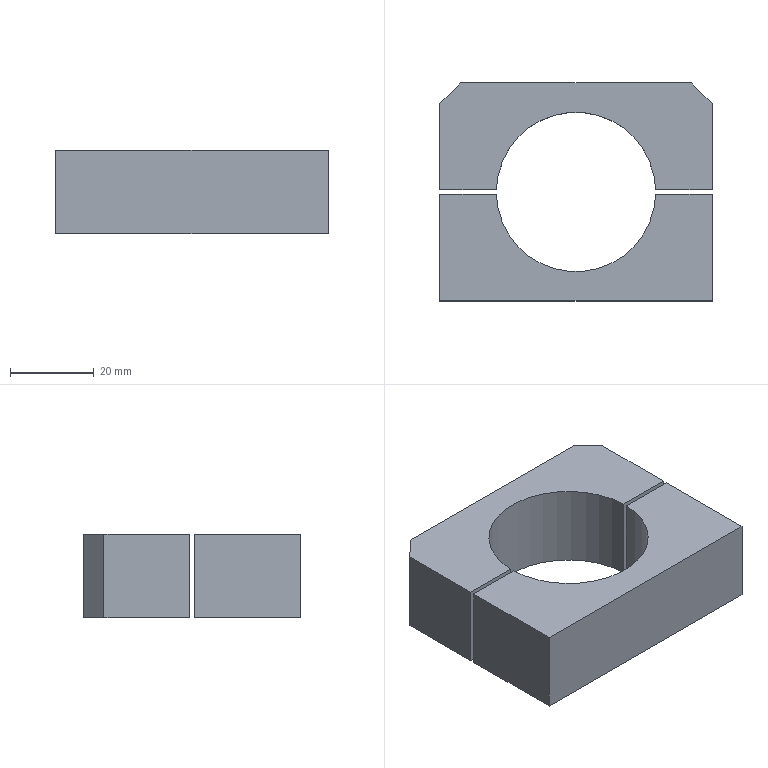Part | STEP file | PN_0008 | 2 solids | 18 faces | box 65 x 52 x 20 mm | volume 43878 mm3 | plane 16 | cylinder 2 | commonest cylinder face diameters 38 x2
STEP:
#1=CARTESIAN_POINT('',(0.,0.,0.));
#2=DIRECTION('',(0.,0.,1.));
#3=DIRECTION('',(1.,0.,0.));
#4=AXIS2_PLACEMENT_3D('',#1,#2,#3);
#5=CARTESIAN_POINT('',(-32.5,-0.5,20.));
#6=VERTEX_POINT('',#5);
#7=CARTESIAN_POINT('',(-18.993,-0.5,20.));
#8=VERTEX_POINT('',#7);
#9=CARTESIAN_POINT('',(-36.358,-0.5,20.));
#10=DIRECTION('',(1.,0.,0.));
#11=VECTOR('',#10,1.);
#12=LINE('',#9,#11);
#13=CARTESIAN_POINT('',(32.5,-26.,20.));
#14=DIRECTION('',(0.,0.,1.));
#15=DIRECTION('',(1.,0.,0.));
#16=AXIS2_PLACEMENT_3D('',#13,#14,#15);
#17=PLANE('',#16);
#18=CARTESIAN_POINT('',(-68.858,25.5));
#19=DIRECTION('',(1.,0.));
#20=VECTOR('',#19,1.);
#21=LINE('',#18,#20);
#22=(GEOMETRIC_REPRESENTATION_CONTEXT(2)PARAMETRIC_REPRESENTATION_CONTEXT()REPRESENTATION_CONTEXT('',''));
#23=DEFINITIONAL_REPRESENTATION('',(#21),#22);
#24=PCURVE('',#17,#23);
#25=CARTESIAN_POINT('',(-36.358,-0.5,0.));
#26=DIRECTION('',(0.,-1.,0.));
#27=DIRECTION('',(0.,0.,-1.));
#28=AXIS2_PLACEMENT_3D('',#25,#26,#27);
#29=PLANE('',#28);
#30=CARTESIAN_POINT('',(-20.,0.));
#31=DIRECTION('',(0.,1.));
#32=VECTOR('',#31,1.);
#33=LINE('',#30,#32);
#34=(GEOMETRIC_REPRESENTATION_CONTEXT(2)PARAMETRIC_REPRESENTATION_CONTEXT()REPRESENTATION_CONTEXT('',''));
#35=DEFINITIONAL_REPRESENTATION('',(#33),#34);
#36=PCURVE('',#29,#35);
#37=SURFACE_CURVE('',#12,(#24,#36),.PCURVE_S1.);
#38=EDGE_CURVE('',#6,#8,#37,.T.);
#39=ORIENTED_EDGE('',*,*,#38,.F.);
#40=CARTESIAN_POINT('',(-32.5,-26.,20.));
#41=VERTEX_POINT('',#40);
#42=CARTESIAN_POINT('',(-32.5,26.,20.));
#43=DIRECTION('',(0.,-1.,0.));
#44=VECTOR('',#43,1.);
#45=LINE('',#42,#44);
#46=CARTESIAN_POINT('',(-65.,52.));
#47=DIRECTION('',(0.,-1.));
#48=VECTOR('',#47,1.);
#49=LINE('',#46,#48);
#50=(GEOMETRIC_REPRESENTATION_CONTEXT(2)PARAMETRIC_REPRESENTATION_CONTEXT()REPRESENTATION_CONTEXT('',''));
#51=DEFINITIONAL_REPRESENTATION('',(#49),#50);
#52=PCURVE('',#17,#51);
#53=CARTESIAN_POINT('',(-32.5,26.,20.));
#54=DIRECTION('',(1.,0.,0.));
#55=DIRECTION('',(0.,1.,0.));
#56=AXIS2_PLACEMENT_3D('',#53,#54,#55);
#57=PLANE('',#56);
#58=CARTESIAN_POINT('',(0.,0.));
#59=DIRECTION('',(-1.,0.));
#60=VECTOR('',#59,1.);
#61=LINE('',#58,#60);
#62=(GEOMETRIC_REPRESENTATION_CONTEXT(2)PARAMETRIC_REPRESENTATION_CONTEXT()REPRESENTATION_CONTEXT('',''));
#63=DEFINITIONAL_REPRESENTATION('',(#61),#62);
#64=PCURVE('',#57,#63);
#65=SURFACE_CURVE('',#45,(#52,#64),.PCURVE_S1.);
#66=EDGE_CURVE('',#6,#41,#65,.T.);
#67=ORIENTED_EDGE('',*,*,#66,.T.);
#68=CARTESIAN_POINT('',(32.5,-26.,20.));
#69=VERTEX_POINT('',#68);
#70=CARTESIAN_POINT('',(-32.5,-26.,20.));
#71=DIRECTION('',(1.,0.,0.));
#72=VECTOR('',#71,1.);
#73=LINE('',#70,#72);
#74=CARTESIAN_POINT('',(-65.,0.));
#75=DIRECTION('',(1.,0.));
#76=VECTOR('',#75,1.);
#77=LINE('',#74,#76);
#78=(GEOMETRIC_REPRESENTATION_CONTEXT(2)PARAMETRIC_REPRESENTATION_CONTEXT()REPRESENTATION_CONTEXT('',''));
#79=DEFINITIONAL_REPRESENTATION('',(#77),#78);
#80=PCURVE('',#17,#79);
#81=CARTESIAN_POINT('',(-32.5,-26.,20.));
#82=DIRECTION('',(0.,1.,0.));
#83=DIRECTION('',(0.,0.,1.));
#84=AXIS2_PLACEMENT_3D('',#81,#82,#83);
#85=PLANE('',#84);
#86=CARTESIAN_POINT('',(0.,0.));
#87=DIRECTION('',(0.,1.));
#88=VECTOR('',#87,1.);
#89=LINE('',#86,#88);
#90=(GEOMETRIC_REPRESENTATION_CONTEXT(2)PARAMETRIC_REPRESENTATION_CONTEXT()REPRESENTATION_CONTEXT('',''));
#91=DEFINITIONAL_REPRESENTATION('',(#89),#90);
#92=PCURVE('',#85,#91);
#93=SURFACE_CURVE('',#73,(#80,#92),.PCURVE_S1.);
#94=EDGE_CURVE('',#41,#69,#93,.T.);
#95=ORIENTED_EDGE('',*,*,#94,.T.);
#96=CARTESIAN_POINT('',(32.5,-0.5,20.));
#97=VERTEX_POINT('',#96);
#98=CARTESIAN_POINT('',(32.5,26.,20.));
#99=DIRECTION('',(0.,1.,0.));
#100=VECTOR('',#99,1.);
#101=LINE('',#98,#100);
#102=CARTESIAN_POINT('',(0.,52.));
#103=DIRECTION('',(0.,1.));
#104=VECTOR('',#103,1.);
#105=LINE('',#102,#104);
#106=(GEOMETRIC_REPRESENTATION_CONTEXT(2)PARAMETRIC_REPRESENTATION_CONTEXT()REPRESENTATION_CONTEXT('',''));
#107=DEFINITIONAL_REPRESENTATION('',(#105),#106);
#108=PCURVE('',#17,#107);
#109=CARTESIAN_POINT('',(32.5,26.,20.));
#110=DIRECTION('',(-1.,0.,0.));
#111=DIRECTION('',(0.,-1.,0.));
#112=AXIS2_PLACEMENT_3D('',#109,#110,#111);
#113=PLANE('',#112);
#114=CARTESIAN_POINT('',(0.,0.));
#115=DIRECTION('',(-1.,0.));
#116=VECTOR('',#115,1.);
#117=LINE('',#114,#116);
#118=(GEOMETRIC_REPRESENTATION_CONTEXT(2)PARAMETRIC_REPRESENTATION_CONTEXT()REPRESENTATION_CONTEXT('',''));
#119=DEFINITIONAL_REPRESENTATION('',(#117),#118);
#120=PCURVE('',#113,#119);
#121=SURFACE_CURVE('',#101,(#108,#120),.PCURVE_S1.);
#122=EDGE_CURVE('',#69,#97,#121,.T.);
#123=ORIENTED_EDGE('',*,*,#122,.T.);
#124=CARTESIAN_POINT('',(18.993,-0.5,20.));
#125=VERTEX_POINT('',#124);
#126=CARTESIAN_POINT('',(-36.358,-0.5,20.));
#127=DIRECTION('',(1.,0.,0.));
#128=VECTOR('',#127,1.);
#129=LINE('',#126,#128);
#130=CARTESIAN_POINT('',(-68.858,25.5));
#131=DIRECTION('',(1.,0.));
#132=VECTOR('',#131,1.);
#133=LINE('',#130,#132);
#134=(GEOMETRIC_REPRESENTATION_CONTEXT(2)PARAMETRIC_REPRESENTATION_CONTEXT()REPRESENTATION_CONTEXT('',''));
#135=DEFINITIONAL_REPRESENTATION('',(#133),#134);
#136=PCURVE('',#17,#135);
#137=CARTESIAN_POINT('',(-36.358,-0.5,0.));
#138=DIRECTION('',(0.,-1.,0.));
#139=DIRECTION('',(0.,0.,-1.));
#140=AXIS2_PLACEMENT_3D('',#137,#138,#139);
#141=PLANE('',#140);
#142=CARTESIAN_POINT('',(-20.,0.));
#143=DIRECTION('',(0.,1.));
#144=VECTOR('',#143,1.);
#145=LINE('',#142,#144);
#146=(GEOMETRIC_REPRESENTATION_CONTEXT(2)PARAMETRIC_REPRESENTATION_CONTEXT()REPRESENTATION_CONTEXT('',''));
#147=DEFINITIONAL_REPRESENTATION('',(#145),#146);
#148=PCURVE('',#141,#147);
#149=SURFACE_CURVE('',#129,(#136,#148),.PCURVE_S1.);
#150=EDGE_CURVE('',#125,#97,#149,.T.);
#151=ORIENTED_EDGE('',*,*,#150,.F.);
#152=CARTESIAN_POINT('',(0.,0.,20.));
#153=DIRECTION('',(0.,0.,1.));
#154=DIRECTION('',(1.,0.,0.));
#155=AXIS2_PLACEMENT_3D('',#152,#153,#154);
#156=CIRCLE('',#155,19.);
#157=CARTESIAN_POINT('',(-32.5,26.));
#158=DIRECTION('',(1.,0.));
#159=AXIS2_PLACEMENT_2D('',#157,#158);
#160=CIRCLE('',#159,19.);
#161=(GEOMETRIC_REPRESENTATION_CONTEXT(2)PARAMETRIC_REPRESENTATION_CONTEXT()REPRESENTATION_CONTEXT('',''));
#162=DEFINITIONAL_REPRESENTATION('',(#160),#161);
#163=PCURVE('',#17,#162);
#164=CARTESIAN_POINT('',(0.,0.,20.));
#165=DIRECTION('',(0.,0.,-1.));
#166=DIRECTION('',(-1.,0.,0.));
#167=AXIS2_PLACEMENT_3D('',#164,#165,#166);
#168=CYLINDRICAL_SURFACE('',#167,19.);
#169=CARTESIAN_POINT('',(9.425,0.));
#170=DIRECTION('',(-1.,0.));
#171=VECTOR('',#170,1.);
#172=LINE('',#169,#171);
#173=(GEOMETRIC_REPRESENTATION_CONTEXT(2)PARAMETRIC_REPRESENTATION_CONTEXT()REPRESENTATION_CONTEXT('',''));
#174=DEFINITIONAL_REPRESENTATION('',(#172),#173);
#175=PCURVE('',#168,#174);
#176=SURFACE_CURVE('',#156,(#163,#175),.PCURVE_S1.);
#177=EDGE_CURVE('',#8,#125,#176,.T.);
#178=ORIENTED_EDGE('',*,*,#177,.F.);
#179=EDGE_LOOP('',(#39,#67,#95,#123,#151,#178));
#180=FACE_BOUND('',#179,.T.);
#181=ADVANCED_FACE('',(#180),#17,.T.);
#182=CARTESIAN_POINT('',(-32.5,-0.5,0.));
#183=VERTEX_POINT('',#182);
#184=CARTESIAN_POINT('',(-32.5,-26.,0.));
#185=VERTEX_POINT('',#184);
#186=CARTESIAN_POINT('',(-32.5,26.,0.));
#187=DIRECTION('',(0.,-1.,0.));
#188=VECTOR('',#187,1.);
#189=LINE('',#186,#188);
#190=CARTESIAN_POINT('',(32.5,-26.,0.));
#191=DIRECTION('',(0.,0.,1.));
#192=DIRECTION('',(1.,0.,0.));
#193=AXIS2_PLACEMENT_3D('',#190,#191,#192);
#194=PLANE('',#193);
#195=CARTESIAN_POINT('',(-65.,52.));
#196=DIRECTION('',(0.,-1.));
#197=VECTOR('',#196,1.);
#198=LINE('',#195,#197);
#199=(GEOMETRIC_REPRESENTATION_CONTEXT(2)PARAMETRIC_REPRESENTATION_CONTEXT()REPRESENTATION_CONTEXT('',''));
#200=DEFINITIONAL_REPRESENTATION('',(#198),#199);
#201=PCURVE('',#194,#200);
#202=CARTESIAN_POINT('',(0.,-20.));
#203=DIRECTION('',(-1.,0.));
#204=VECTOR('',#203,1.);
#205=LINE('',#202,#204);
#206=(GEOMETRIC_REPRESENTATION_CONTEXT(2)PARAMETRIC_REPRESENTATION_CONTEXT()REPRESENTATION_CONTEXT('',''));
#207=DEFINITIONAL_REPRESENTATION('',(#205),#206);
#208=PCURVE('',#57,#207);
#209=SURFACE_CURVE('',#189,(#201,#208),.PCURVE_S1.);
#210=EDGE_CURVE('',#183,#185,#209,.T.);
#211=ORIENTED_EDGE('',*,*,#210,.F.);
#212=CARTESIAN_POINT('',(-18.993,-0.5,0.));
#213=VERTEX_POINT('',#212);
#214=CARTESIAN_POINT('',(-36.358,-0.5,0.));
#215=DIRECTION('',(1.,0.,0.));
#216=VECTOR('',#215,1.);
#217=LINE('',#214,#216);
#218=CARTESIAN_POINT('',(-68.858,25.5));
#219=DIRECTION('',(1.,0.));
#220=VECTOR('',#219,1.);
#221=LINE('',#218,#220);
#222=(GEOMETRIC_REPRESENTATION_CONTEXT(2)PARAMETRIC_REPRESENTATION_CONTEXT()REPRESENTATION_CONTEXT('',''));
#223=DEFINITIONAL_REPRESENTATION('',(#221),#222);
#224=PCURVE('',#194,#223);
#225=CARTESIAN_POINT('',(0.,0.));
#226=DIRECTION('',(0.,1.));
#227=VECTOR('',#226,1.);
#228=LINE('',#225,#227);
#229=(GEOMETRIC_REPRESENTATION_CONTEXT(2)PARAMETRIC_REPRESENTATION_CONTEXT()REPRESENTATION_CONTEXT('',''));
#230=DEFINITIONAL_REPRESENTATION('',(#228),#229);
#231=PCURVE('',#29,#230);
#232=SURFACE_CURVE('',#217,(#224,#231),.PCURVE_S1.);
#233=EDGE_CURVE('',#183,#213,#232,.T.);
#234=ORIENTED_EDGE('',*,*,#233,.T.);
#235=CARTESIAN_POINT('',(18.993,-0.5,0.));
#236=VERTEX_POINT('',#235);
#237=CARTESIAN_POINT('',(0.,0.,0.));
#238=DIRECTION('',(0.,0.,1.));
#239=DIRECTION('',(1.,0.,0.));
#240=AXIS2_PLACEMENT_3D('',#237,#238,#239);
#241=CIRCLE('',#240,19.);
#242=CARTESIAN_POINT('',(-32.5,26.));
#243=DIRECTION('',(1.,0.));
#244=AXIS2_PLACEMENT_2D('',#242,#243);
#245=CIRCLE('',#244,19.);
#246=(GEOMETRIC_REPRESENTATION_CONTEXT(2)PARAMETRIC_REPRESENTATION_CONTEXT()REPRESENTATION_CONTEXT('',''));
#247=DEFINITIONAL_REPRESENTATION('',(#245),#246);
#248=PCURVE('',#194,#247);
#249=CARTESIAN_POINT('',(9.425,20.));
#250=DIRECTION('',(-1.,0.));
#251=VECTOR('',#250,1.);
#252=LINE('',#249,#251);
#253=(GEOMETRIC_REPRESENTATION_CONTEXT(2)PARAMETRIC_REPRESENTATION_CONTEXT()REPRESENTATION_CONTEXT('',''));
#254=DEFINITIONAL_REPRESENTATION('',(#252),#253);
#255=PCURVE('',#168,#254);
#256=SURFACE_CURVE('',#241,(#248,#255),.PCURVE_S1.);
#257=EDGE_CURVE('',#213,#236,#256,.T.);
#258=ORIENTED_EDGE('',*,*,#257,.T.);
#259=CARTESIAN_POINT('',(32.5,-0.5,0.));
#260=VERTEX_POINT('',#259);
#261=CARTESIAN_POINT('',(-36.358,-0.5,0.));
#262=DIRECTION('',(1.,0.,0.));
#263=VECTOR('',#262,1.);
#264=LINE('',#261,#263);
#265=CARTESIAN_POINT('',(-68.858,25.5));
#266=DIRECTION('',(1.,0.));
#267=VECTOR('',#266,1.);
#268=LINE('',#265,#267);
#269=(GEOMETRIC_REPRESENTATION_CONTEXT(2)PARAMETRIC_REPRESENTATION_CONTEXT()REPRESENTATION_CONTEXT('',''));
#270=DEFINITIONAL_REPRESENTATION('',(#268),#269);
#271=PCURVE('',#194,#270);
#272=CARTESIAN_POINT('',(0.,0.));
#273=DIRECTION('',(0.,1.));
#274=VECTOR('',#273,1.);
#275=LINE('',#272,#274);
#276=(GEOMETRIC_REPRESENTATION_CONTEXT(2)PARAMETRIC_REPRESENTATION_CONTEXT()REPRESENTATION_CONTEXT('',''));
#277=DEFINITIONAL_REPRESENTATION('',(#275),#276);
#278=PCURVE('',#141,#277);
#279=SURFACE_CURVE('',#264,(#271,#278),.PCURVE_S1.);
#280=EDGE_CURVE('',#236,#260,#279,.T.);
#281=ORIENTED_EDGE('',*,*,#280,.T.);
#282=CARTESIAN_POINT('',(32.5,-26.,0.));
#283=VERTEX_POINT('',#282);
#284=CARTESIAN_POINT('',(32.5,26.,0.));
#285=DIRECTION('',(0.,1.,0.));
#286=VECTOR('',#285,1.);
#287=LINE('',#284,#286);
#288=CARTESIAN_POINT('',(0.,52.));
#289=DIRECTION('',(0.,1.));
#290=VECTOR('',#289,1.);
#291=LINE('',#288,#290);
#292=(GEOMETRIC_REPRESENTATION_CONTEXT(2)PARAMETRIC_REPRESENTATION_CONTEXT()REPRESENTATION_CONTEXT('',''));
#293=DEFINITIONAL_REPRESENTATION('',(#291),#292);
#294=PCURVE('',#194,#293);
#295=CARTESIAN_POINT('',(0.,-20.));
#296=DIRECTION('',(-1.,0.));
#297=VECTOR('',#296,1.);
#298=LINE('',#295,#297);
#299=(GEOMETRIC_REPRESENTATION_CONTEXT(2)PARAMETRIC_REPRESENTATION_CONTEXT()REPRESENTATION_CONTEXT('',''));
#300=DEFINITIONAL_REPRESENTATION('',(#298),#299);
#301=PCURVE('',#113,#300);
#302=SURFACE_CURVE('',#287,(#294,#301),.PCURVE_S1.);
#303=EDGE_CURVE('',#283,#260,#302,.T.);
#304=ORIENTED_EDGE('',*,*,#303,.F.);
#305=CARTESIAN_POINT('',(-32.5,-26.,0.));
#306=DIRECTION('',(1.,0.,0.));
#307=VECTOR('',#306,1.);
#308=LINE('',#305,#307);
#309=CARTESIAN_POINT('',(-65.,0.));
#310=DIRECTION('',(1.,0.));
#311=VECTOR('',#310,1.);
#312=LINE('',#309,#311);
#313=(GEOMETRIC_REPRESENTATION_CONTEXT(2)PARAMETRIC_REPRESENTATION_CONTEXT()REPRESENTATION_CONTEXT('',''));
#314=DEFINITIONAL_REPRESENTATION('',(#312),#313);
#315=PCURVE('',#194,#314);
#316=CARTESIAN_POINT('',(-20.,0.));
#317=DIRECTION('',(0.,1.));
#318=VECTOR('',#317,1.);
#319=LINE('',#316,#318);
#320=(GEOMETRIC_REPRESENTATION_CONTEXT(2)PARAMETRIC_REPRESENTATION_CONTEXT()REPRESENTATION_CONTEXT('',''));
#321=DEFINITIONAL_REPRESENTATION('',(#319),#320);
#322=PCURVE('',#85,#321);
#323=SURFACE_CURVE('',#308,(#315,#322),.PCURVE_S1.);
#324=EDGE_CURVE('',#185,#283,#323,.T.);
#325=ORIENTED_EDGE('',*,*,#324,.F.);
#326=EDGE_LOOP('',(#211,#234,#258,#281,#304,#325));
#327=FACE_BOUND('',#326,.T.);
#328=ADVANCED_FACE('',(#327),#194,.F.);
#329=ORIENTED_EDGE('',*,*,#303,.T.);
#330=CARTESIAN_POINT('',(32.5,-0.5,20.));
#331=DIRECTION('',(0.,0.,1.));
#332=VECTOR('',#331,1.);
#333=LINE('',#330,#332);
#334=CARTESIAN_POINT('',(26.5,0.));
#335=DIRECTION('',(0.,1.));
#336=VECTOR('',#335,1.);
#337=LINE('',#334,#336);
#338=(GEOMETRIC_REPRESENTATION_CONTEXT(2)PARAMETRIC_REPRESENTATION_CONTEXT()REPRESENTATION_CONTEXT('',''));
#339=DEFINITIONAL_REPRESENTATION('',(#337),#338);
#340=PCURVE('',#113,#339);
#341=CARTESIAN_POINT('',(-20.,68.858));
#342=DIRECTION('',(-1.,0.));
#343=VECTOR('',#342,1.);
#344=LINE('',#341,#343);
#345=(GEOMETRIC_REPRESENTATION_CONTEXT(2)PARAMETRIC_REPRESENTATION_CONTEXT()REPRESENTATION_CONTEXT('',''));
#346=DEFINITIONAL_REPRESENTATION('',(#344),#345);
#347=PCURVE('',#141,#346);
#348=SURFACE_CURVE('',#333,(#340,#347),.PCURVE_S1.);
#349=EDGE_CURVE('',#260,#97,#348,.T.);
#350=ORIENTED_EDGE('',*,*,#349,.T.);
#351=ORIENTED_EDGE('',*,*,#122,.F.);
#352=CARTESIAN_POINT('',(32.5,-26.,20.));
#353=DIRECTION('',(0.,0.,-1.));
#354=VECTOR('',#353,1.);
#355=LINE('',#352,#354);
#356=CARTESIAN_POINT('',(52.,0.));
#357=DIRECTION('',(0.,-1.));
#358=VECTOR('',#357,1.);
#359=LINE('',#356,#358);
#360=(GEOMETRIC_REPRESENTATION_CONTEXT(2)PARAMETRIC_REPRESENTATION_CONTEXT()REPRESENTATION_CONTEXT('',''));
#361=DEFINITIONAL_REPRESENTATION('',(#359),#360);
#362=PCURVE('',#113,#361);
#363=CARTESIAN_POINT('',(0.,65.));
#364=DIRECTION('',(-1.,0.));
#365=VECTOR('',#364,1.);
#366=LINE('',#363,#365);
#367=(GEOMETRIC_REPRESENTATION_CONTEXT(2)PARAMETRIC_REPRESENTATION_CONTEXT()REPRESENTATION_CONTEXT('',''));
#368=DEFINITIONAL_REPRESENTATION('',(#366),#367);
#369=PCURVE('',#85,#368);
#370=SURFACE_CURVE('',#355,(#362,#369),.PCURVE_S1.);
#371=EDGE_CURVE('',#69,#283,#370,.T.);
#372=ORIENTED_EDGE('',*,*,#371,.T.);
#373=EDGE_LOOP('',(#329,#350,#351,#372));
#374=FACE_BOUND('',#373,.T.);
#375=ADVANCED_FACE('',(#374),#113,.F.);
#376=ORIENTED_EDGE('',*,*,#66,.F.);
#377=CARTESIAN_POINT('',(-32.5,-0.5,20.));
#378=DIRECTION('',(0.,0.,-1.));
#379=VECTOR('',#378,1.);
#380=LINE('',#377,#379);
#381=CARTESIAN_POINT('',(-26.5,0.));
#382=DIRECTION('',(0.,-1.));
#383=VECTOR('',#382,1.);
#384=LINE('',#381,#383);
#385=(GEOMETRIC_REPRESENTATION_CONTEXT(2)PARAMETRIC_REPRESENTATION_CONTEXT()REPRESENTATION_CONTEXT('',''));
#386=DEFINITIONAL_REPRESENTATION('',(#384),#385);
#387=PCURVE('',#57,#386);
#388=CARTESIAN_POINT('',(-20.,3.858));
#389=DIRECTION('',(1.,0.));
#390=VECTOR('',#389,1.);
#391=LINE('',#388,#390);
#392=(GEOMETRIC_REPRESENTATION_CONTEXT(2)PARAMETRIC_REPRESENTATION_CONTEXT()REPRESENTATION_CONTEXT('',''));
#393=DEFINITIONAL_REPRESENTATION('',(#391),#392);
#394=PCURVE('',#29,#393);
#395=SURFACE_CURVE('',#380,(#387,#394),.PCURVE_S1.);
#396=EDGE_CURVE('',#6,#183,#395,.T.);
#397=ORIENTED_EDGE('',*,*,#396,.T.);
#398=ORIENTED_EDGE('',*,*,#210,.T.);
#399=CARTESIAN_POINT('',(-32.5,-26.,20.));
#400=DIRECTION('',(0.,0.,-1.));
#401=VECTOR('',#400,1.);
#402=LINE('',#399,#401);
#403=CARTESIAN_POINT('',(-52.,0.));
#404=DIRECTION('',(0.,-1.));
#405=VECTOR('',#404,1.);
#406=LINE('',#403,#405);
#407=(GEOMETRIC_REPRESENTATION_CONTEXT(2)PARAMETRIC_REPRESENTATION_CONTEXT()REPRESENTATION_CONTEXT('',''));
#408=DEFINITIONAL_REPRESENTATION('',(#406),#407);
#409=PCURVE('',#57,#408);
#410=CARTESIAN_POINT('',(0.,0.));
#411=DIRECTION('',(-1.,0.));
#412=VECTOR('',#411,1.);
#413=LINE('',#410,#412);
#414=(GEOMETRIC_REPRESENTATION_CONTEXT(2)PARAMETRIC_REPRESENTATION_CONTEXT()REPRESENTATION_CONTEXT('',''));
#415=DEFINITIONAL_REPRESENTATION('',(#413),#414);
#416=PCURVE('',#85,#415);
#417=SURFACE_CURVE('',#402,(#409,#416),.PCURVE_S1.);
#418=EDGE_CURVE('',#41,#185,#417,.T.);
#419=ORIENTED_EDGE('',*,*,#418,.F.);
#420=EDGE_LOOP('',(#376,#397,#398,#419));
#421=FACE_BOUND('',#420,.T.);
#422=ADVANCED_FACE('',(#421),#57,.F.);
#423=ORIENTED_EDGE('',*,*,#257,.T.);
#424=CARTESIAN_POINT('',(18.993,-0.5,20.));
#425=DIRECTION('',(0.,0.,1.));
#426=VECTOR('',#425,1.);
#427=LINE('',#424,#426);
#428=CARTESIAN_POINT('',(3.168,0.));
#429=DIRECTION('',(0.,-1.));
#430=VECTOR('',#429,1.);
#431=LINE('',#428,#430);
#432=(GEOMETRIC_REPRESENTATION_CONTEXT(2)PARAMETRIC_REPRESENTATION_CONTEXT()REPRESENTATION_CONTEXT('',''));
#433=DEFINITIONAL_REPRESENTATION('',(#431),#432);
#434=PCURVE('',#168,#433);
#435=CARTESIAN_POINT('',(-20.,55.352));
#436=DIRECTION('',(-1.,0.));
#437=VECTOR('',#436,1.);
#438=LINE('',#435,#437);
#439=(GEOMETRIC_REPRESENTATION_CONTEXT(2)PARAMETRIC_REPRESENTATION_CONTEXT()REPRESENTATION_CONTEXT('',''));
#440=DEFINITIONAL_REPRESENTATION('',(#438),#439);
#441=PCURVE('',#141,#440);
#442=SURFACE_CURVE('',#427,(#434,#441),.PCURVE_S1.);
#443=EDGE_CURVE('',#236,#125,#442,.T.);
#444=ORIENTED_EDGE('',*,*,#443,.T.);
#445=ORIENTED_EDGE('',*,*,#177,.F.);
#446=CARTESIAN_POINT('',(-18.993,-0.5,20.));
#447=DIRECTION('',(0.,0.,-1.));
#448=VECTOR('',#447,1.);
#449=LINE('',#446,#448);
#450=CARTESIAN_POINT('',(6.257,0.));
#451=DIRECTION('',(0.,1.));
#452=VECTOR('',#451,1.);
#453=LINE('',#450,#452);
#454=(GEOMETRIC_REPRESENTATION_CONTEXT(2)PARAMETRIC_REPRESENTATION_CONTEXT()REPRESENTATION_CONTEXT('',''));
#455=DEFINITIONAL_REPRESENTATION('',(#453),#454);
#456=PCURVE('',#168,#455);
#457=CARTESIAN_POINT('',(-20.,17.365));
#458=DIRECTION('',(1.,0.));
#459=VECTOR('',#458,1.);
#460=LINE('',#457,#459);
#461=(GEOMETRIC_REPRESENTATION_CONTEXT(2)PARAMETRIC_REPRESENTATION_CONTEXT()REPRESENTATION_CONTEXT('',''));
#462=DEFINITIONAL_REPRESENTATION('',(#460),#461);
#463=PCURVE('',#29,#462);
#464=SURFACE_CURVE('',#449,(#456,#463),.PCURVE_S1.);
#465=EDGE_CURVE('',#8,#213,#464,.T.);
#466=ORIENTED_EDGE('',*,*,#465,.T.);
#467=EDGE_LOOP('',(#423,#444,#445,#466));
#468=FACE_BOUND('',#467,.F.);
#469=ADVANCED_FACE('',(#468),#168,.F.);
#470=ORIENTED_EDGE('',*,*,#324,.T.);
#471=ORIENTED_EDGE('',*,*,#371,.F.);
#472=ORIENTED_EDGE('',*,*,#94,.F.);
#473=ORIENTED_EDGE('',*,*,#418,.T.);
#474=EDGE_LOOP('',(#470,#471,#472,#473));
#475=FACE_BOUND('',#474,.T.);
#476=ADVANCED_FACE('',(#475),#85,.F.);
#477=ORIENTED_EDGE('',*,*,#280,.F.);
#478=ORIENTED_EDGE('',*,*,#443,.T.);
#479=ORIENTED_EDGE('',*,*,#150,.T.);
#480=ORIENTED_EDGE('',*,*,#349,.F.);
#481=EDGE_LOOP('',(#477,#478,#479,#480));
#482=FACE_BOUND('',#481,.T.);
#483=ADVANCED_FACE('',(#482),#141,.F.);
#484=ORIENTED_EDGE('',*,*,#38,.T.);
#485=ORIENTED_EDGE('',*,*,#465,.T.);
#486=ORIENTED_EDGE('',*,*,#233,.F.);
#487=ORIENTED_EDGE('',*,*,#396,.F.);
#488=EDGE_LOOP('',(#484,#485,#486,#487));
#489=FACE_BOUND('',#488,.T.);
#490=ADVANCED_FACE('',(#489),#29,.F.);
#491=CLOSED_SHELL('',(#181,#328,#375,#422,#469,#476,#483,#490));
#492=MANIFOLD_SOLID_BREP('',#491);
#493=CARTESIAN_POINT('',(27.5,26.,20.));
#494=VERTEX_POINT('',#493);
#495=CARTESIAN_POINT('',(-27.5,26.,20.));
#496=VERTEX_POINT('',#495);
#497=CARTESIAN_POINT('',(-32.5,26.,20.));
#498=DIRECTION('',(-1.,0.,0.));
#499=VECTOR('',#498,1.);
#500=LINE('',#497,#499);
#501=CARTESIAN_POINT('',(-32.5,26.,20.));
#502=DIRECTION('',(0.,-1.,0.));
#503=DIRECTION('',(0.,0.,-1.));
#504=AXIS2_PLACEMENT_3D('',#501,#502,#503);
#505=PLANE('',#504);
#506=CARTESIAN_POINT('',(0.,0.));
#507=DIRECTION('',(0.,-1.));
#508=VECTOR('',#507,1.);
#509=LINE('',#506,#508);
#510=(GEOMETRIC_REPRESENTATION_CONTEXT(2)PARAMETRIC_REPRESENTATION_CONTEXT()REPRESENTATION_CONTEXT('',''));
#511=DEFINITIONAL_REPRESENTATION('',(#509),#510);
#512=PCURVE('',#505,#511);
#513=CARTESIAN_POINT('',(32.5,-26.,20.));
#514=DIRECTION('',(0.,0.,1.));
#515=DIRECTION('',(1.,0.,0.));
#516=AXIS2_PLACEMENT_3D('',#513,#514,#515);
#517=PLANE('',#516);
#518=CARTESIAN_POINT('',(-65.,52.));
#519=DIRECTION('',(-1.,0.));
#520=VECTOR('',#519,1.);
#521=LINE('',#518,#520);
#522=(GEOMETRIC_REPRESENTATION_CONTEXT(2)PARAMETRIC_REPRESENTATION_CONTEXT()REPRESENTATION_CONTEXT('',''));
#523=DEFINITIONAL_REPRESENTATION('',(#521),#522);
#524=PCURVE('',#517,#523);
#525=SURFACE_CURVE('',#500,(#512,#524),.PCURVE_S1.);
#526=EDGE_CURVE('',#494,#496,#525,.T.);
#527=ORIENTED_EDGE('',*,*,#526,.F.);
#528=CARTESIAN_POINT('',(27.5,26.,0.));
#529=VERTEX_POINT('',#528);
#530=CARTESIAN_POINT('',(27.5,26.,20.));
#531=DIRECTION('',(0.,0.,-1.));
#532=VECTOR('',#531,1.);
#533=LINE('',#530,#532);
#534=CARTESIAN_POINT('',(0.,60.));
#535=DIRECTION('',(1.,0.));
#536=VECTOR('',#535,1.);
#537=LINE('',#534,#536);
#538=(GEOMETRIC_REPRESENTATION_CONTEXT(2)PARAMETRIC_REPRESENTATION_CONTEXT()REPRESENTATION_CONTEXT('',''));
#539=DEFINITIONAL_REPRESENTATION('',(#537),#538);
#540=PCURVE('',#505,#539);
#541=CARTESIAN_POINT('',(27.5,26.,20.));
#542=DIRECTION('',(-0.7071,-0.7071,0.));
#543=DIRECTION('',(0.7071,-0.7071,0.));
#544=AXIS2_PLACEMENT_3D('',#541,#542,#543);
#545=PLANE('',#544);
#546=CARTESIAN_POINT('',(0.,0.));
#547=DIRECTION('',(0.,-1.));
#548=VECTOR('',#547,1.);
#549=LINE('',#546,#548);
#550=(GEOMETRIC_REPRESENTATION_CONTEXT(2)PARAMETRIC_REPRESENTATION_CONTEXT()REPRESENTATION_CONTEXT('',''));
#551=DEFINITIONAL_REPRESENTATION('',(#549),#550);
#552=PCURVE('',#545,#551);
#553=SURFACE_CURVE('',#533,(#540,#552),.PCURVE_S1.);
#554=EDGE_CURVE('',#494,#529,#553,.T.);
#555=ORIENTED_EDGE('',*,*,#554,.T.);
#556=CARTESIAN_POINT('',(-27.5,26.,0.));
#557=VERTEX_POINT('',#556);
#558=CARTESIAN_POINT('',(-32.5,26.,0.));
#559=DIRECTION('',(-1.,0.,0.));
#560=VECTOR('',#559,1.);
#561=LINE('',#558,#560);
#562=CARTESIAN_POINT('',(20.,0.));
#563=DIRECTION('',(0.,-1.));
#564=VECTOR('',#563,1.);
#565=LINE('',#562,#564);
#566=(GEOMETRIC_REPRESENTATION_CONTEXT(2)PARAMETRIC_REPRESENTATION_CONTEXT()REPRESENTATION_CONTEXT('',''));
#567=DEFINITIONAL_REPRESENTATION('',(#565),#566);
#568=PCURVE('',#505,#567);
#569=CARTESIAN_POINT('',(32.5,-26.,0.));
#570=DIRECTION('',(0.,0.,1.));
#571=DIRECTION('',(1.,0.,0.));
#572=AXIS2_PLACEMENT_3D('',#569,#570,#571);
#573=PLANE('',#572);
#574=CARTESIAN_POINT('',(-65.,52.));
#575=DIRECTION('',(-1.,0.));
#576=VECTOR('',#575,1.);
#577=LINE('',#574,#576);
#578=(GEOMETRIC_REPRESENTATION_CONTEXT(2)PARAMETRIC_REPRESENTATION_CONTEXT()REPRESENTATION_CONTEXT('',''));
#579=DEFINITIONAL_REPRESENTATION('',(#577),#578);
#580=PCURVE('',#573,#579);
#581=SURFACE_CURVE('',#561,(#568,#580),.PCURVE_S1.);
#582=EDGE_CURVE('',#529,#557,#581,.T.);
#583=ORIENTED_EDGE('',*,*,#582,.T.);
#584=CARTESIAN_POINT('',(-27.5,26.,20.));
#585=DIRECTION('',(0.,0.,1.));
#586=VECTOR('',#585,1.);
#587=LINE('',#584,#586);
#588=CARTESIAN_POINT('',(0.,5.));
#589=DIRECTION('',(-1.,0.));
#590=VECTOR('',#589,1.);
#591=LINE('',#588,#590);
#592=(GEOMETRIC_REPRESENTATION_CONTEXT(2)PARAMETRIC_REPRESENTATION_CONTEXT()REPRESENTATION_CONTEXT('',''));
#593=DEFINITIONAL_REPRESENTATION('',(#591),#592);
#594=PCURVE('',#505,#593);
#595=CARTESIAN_POINT('',(-32.5,21.,20.));
#596=DIRECTION('',(0.7071,-0.7071,0.));
#597=DIRECTION('',(0.7071,0.7071,0.));
#598=AXIS2_PLACEMENT_3D('',#595,#596,#597);
#599=PLANE('',#598);
#600=CARTESIAN_POINT('',(7.071,0.));
#601=DIRECTION('',(0.,1.));
#602=VECTOR('',#601,1.);
#603=LINE('',#600,#602);
#604=(GEOMETRIC_REPRESENTATION_CONTEXT(2)PARAMETRIC_REPRESENTATION_CONTEXT()REPRESENTATION_CONTEXT('',''));
#605=DEFINITIONAL_REPRESENTATION('',(#603),#604);
#606=PCURVE('',#599,#605);
#607=SURFACE_CURVE('',#587,(#594,#606),.PCURVE_S1.);
#608=EDGE_CURVE('',#557,#496,#607,.T.);
#609=ORIENTED_EDGE('',*,*,#608,.T.);
#610=EDGE_LOOP('',(#527,#555,#583,#609));
#611=FACE_BOUND('',#610,.T.);
#612=ADVANCED_FACE('',(#611),#505,.F.);
#613=CARTESIAN_POINT('',(-32.5,21.,20.));
#614=VERTEX_POINT('',#613);
#615=CARTESIAN_POINT('',(-32.5,0.5,20.));
#616=VERTEX_POINT('',#615);
#617=CARTESIAN_POINT('',(-32.5,26.,20.));
#618=DIRECTION('',(0.,-1.,0.));
#619=VECTOR('',#618,1.);
#620=LINE('',#617,#619);
#621=CARTESIAN_POINT('',(-32.5,26.,20.));
#622=DIRECTION('',(1.,0.,0.));
#623=DIRECTION('',(0.,1.,0.));
#624=AXIS2_PLACEMENT_3D('',#621,#622,#623);
#625=PLANE('',#624);
#626=CARTESIAN_POINT('',(0.,0.));
#627=DIRECTION('',(-1.,0.));
#628=VECTOR('',#627,1.);
#629=LINE('',#626,#628);
#630=(GEOMETRIC_REPRESENTATION_CONTEXT(2)PARAMETRIC_REPRESENTATION_CONTEXT()REPRESENTATION_CONTEXT('',''));
#631=DEFINITIONAL_REPRESENTATION('',(#629),#630);
#632=PCURVE('',#625,#631);
#633=CARTESIAN_POINT('',(-65.,52.));
#634=DIRECTION('',(0.,-1.));
#635=VECTOR('',#634,1.);
#636=LINE('',#633,#635);
#637=(GEOMETRIC_REPRESENTATION_CONTEXT(2)PARAMETRIC_REPRESENTATION_CONTEXT()REPRESENTATION_CONTEXT('',''));
#638=DEFINITIONAL_REPRESENTATION('',(#636),#637);
#639=PCURVE('',#517,#638);
#640=SURFACE_CURVE('',#620,(#632,#639),.PCURVE_S1.);
#641=EDGE_CURVE('',#614,#616,#640,.T.);
#642=ORIENTED_EDGE('',*,*,#641,.F.);
#643=CARTESIAN_POINT('',(-32.5,21.,0.));
#644=VERTEX_POINT('',#643);
#645=CARTESIAN_POINT('',(-32.5,21.,20.));
#646=DIRECTION('',(0.,0.,-1.));
#647=VECTOR('',#646,1.);
#648=LINE('',#645,#647);
#649=CARTESIAN_POINT('',(-5.,0.));
#650=DIRECTION('',(0.,-1.));
#651=VECTOR('',#650,1.);
#652=LINE('',#649,#651);
#653=(GEOMETRIC_REPRESENTATION_CONTEXT(2)PARAMETRIC_REPRESENTATION_CONTEXT()REPRESENTATION_CONTEXT('',''));
#654=DEFINITIONAL_REPRESENTATION('',(#652),#653);
#655=PCURVE('',#625,#654);
#656=CARTESIAN_POINT('',(0.,0.));
#657=DIRECTION('',(0.,-1.));
#658=VECTOR('',#657,1.);
#659=LINE('',#656,#658);
#660=(GEOMETRIC_REPRESENTATION_CONTEXT(2)PARAMETRIC_REPRESENTATION_CONTEXT()REPRESENTATION_CONTEXT('',''));
#661=DEFINITIONAL_REPRESENTATION('',(#659),#660);
#662=PCURVE('',#599,#661);
#663=SURFACE_CURVE('',#648,(#655,#662),.PCURVE_S1.);
#664=EDGE_CURVE('',#614,#644,#663,.T.);
#665=ORIENTED_EDGE('',*,*,#664,.T.);
#666=CARTESIAN_POINT('',(-32.5,0.5,0.));
#667=VERTEX_POINT('',#666);
#668=CARTESIAN_POINT('',(-32.5,26.,0.));
#669=DIRECTION('',(0.,-1.,0.));
#670=VECTOR('',#669,1.);
#671=LINE('',#668,#670);
#672=CARTESIAN_POINT('',(0.,-20.));
#673=DIRECTION('',(-1.,0.));
#674=VECTOR('',#673,1.);
#675=LINE('',#672,#674);
#676=(GEOMETRIC_REPRESENTATION_CONTEXT(2)PARAMETRIC_REPRESENTATION_CONTEXT()REPRESENTATION_CONTEXT('',''));
#677=DEFINITIONAL_REPRESENTATION('',(#675),#676);
#678=PCURVE('',#625,#677);
#679=CARTESIAN_POINT('',(-65.,52.));
#680=DIRECTION('',(0.,-1.));
#681=VECTOR('',#680,1.);
#682=LINE('',#679,#681);
#683=(GEOMETRIC_REPRESENTATION_CONTEXT(2)PARAMETRIC_REPRESENTATION_CONTEXT()REPRESENTATION_CONTEXT('',''));
#684=DEFINITIONAL_REPRESENTATION('',(#682),#683);
#685=PCURVE('',#573,#684);
#686=SURFACE_CURVE('',#671,(#678,#685),.PCURVE_S1.);
#687=EDGE_CURVE('',#644,#667,#686,.T.);
#688=ORIENTED_EDGE('',*,*,#687,.T.);
#689=CARTESIAN_POINT('',(-32.5,0.5,20.));
#690=DIRECTION('',(0.,0.,1.));
#691=VECTOR('',#690,1.);
#692=LINE('',#689,#691);
#693=CARTESIAN_POINT('',(-25.5,0.));
#694=DIRECTION('',(0.,1.));
#695=VECTOR('',#694,1.);
#696=LINE('',#693,#695);
#697=(GEOMETRIC_REPRESENTATION_CONTEXT(2)PARAMETRIC_REPRESENTATION_CONTEXT()REPRESENTATION_CONTEXT('',''));
#698=DEFINITIONAL_REPRESENTATION('',(#696),#697);
#699=PCURVE('',#625,#698);
#700=CARTESIAN_POINT('',(-36.358,0.5,0.));
#701=DIRECTION('',(0.,1.,0.));
#702=DIRECTION('',(0.,0.,1.));
#703=AXIS2_PLACEMENT_3D('',#700,#701,#702);
#704=PLANE('',#703);
#705=CARTESIAN_POINT('',(20.,3.858));
#706=DIRECTION('',(1.,0.));
#707=VECTOR('',#706,1.);
#708=LINE('',#705,#707);
#709=(GEOMETRIC_REPRESENTATION_CONTEXT(2)PARAMETRIC_REPRESENTATION_CONTEXT()REPRESENTATION_CONTEXT('',''));
#710=DEFINITIONAL_REPRESENTATION('',(#708),#709);
#711=PCURVE('',#704,#710);
#712=SURFACE_CURVE('',#692,(#699,#711),.PCURVE_S1.);
#713=EDGE_CURVE('',#667,#616,#712,.T.);
#714=ORIENTED_EDGE('',*,*,#713,.T.);
#715=EDGE_LOOP('',(#642,#665,#688,#714));
#716=FACE_BOUND('',#715,.T.);
#717=ADVANCED_FACE('',(#716),#625,.F.);
#718=CARTESIAN_POINT('',(18.993,0.5,0.));
#719=VERTEX_POINT('',#718);
#720=CARTESIAN_POINT('',(-18.993,0.5,0.));
#721=VERTEX_POINT('',#720);
#722=CARTESIAN_POINT('',(0.,0.,0.));
#723=DIRECTION('',(0.,0.,1.));
#724=DIRECTION('',(1.,0.,0.));
#725=AXIS2_PLACEMENT_3D('',#722,#723,#724);
#726=CIRCLE('',#725,19.);
#727=CARTESIAN_POINT('',(0.,0.,20.));
#728=DIRECTION('',(0.,0.,-1.));
#729=DIRECTION('',(-1.,0.,0.));
#730=AXIS2_PLACEMENT_3D('',#727,#728,#729);
#731=CYLINDRICAL_SURFACE('',#730,19.);
#732=CARTESIAN_POINT('',(3.142,20.));
#733=DIRECTION('',(-1.,0.));
#734=VECTOR('',#733,1.);
#735=LINE('',#732,#734);
#736=(GEOMETRIC_REPRESENTATION_CONTEXT(2)PARAMETRIC_REPRESENTATION_CONTEXT()REPRESENTATION_CONTEXT('',''));
#737=DEFINITIONAL_REPRESENTATION('',(#735),#736);
#738=PCURVE('',#731,#737);
#739=CARTESIAN_POINT('',(-32.5,26.));
#740=DIRECTION('',(1.,0.));
#741=AXIS2_PLACEMENT_2D('',#739,#740);
#742=CIRCLE('',#741,19.);
#743=(GEOMETRIC_REPRESENTATION_CONTEXT(2)PARAMETRIC_REPRESENTATION_CONTEXT()REPRESENTATION_CONTEXT('',''));
#744=DEFINITIONAL_REPRESENTATION('',(#742),#743);
#745=PCURVE('',#573,#744);
#746=SURFACE_CURVE('',#726,(#738,#745),.PCURVE_S1.);
#747=EDGE_CURVE('',#719,#721,#746,.T.);
#748=ORIENTED_EDGE('',*,*,#747,.T.);
#749=CARTESIAN_POINT('',(-18.993,0.5,20.));
#750=VERTEX_POINT('',#749);
#751=CARTESIAN_POINT('',(-18.993,0.5,20.));
#752=DIRECTION('',(0.,0.,1.));
#753=VECTOR('',#752,1.);
#754=LINE('',#751,#753);
#755=CARTESIAN_POINT('',(0.02632,0.));
#756=DIRECTION('',(0.,-1.));
#757=VECTOR('',#756,1.);
#758=LINE('',#755,#757);
#759=(GEOMETRIC_REPRESENTATION_CONTEXT(2)PARAMETRIC_REPRESENTATION_CONTEXT()REPRESENTATION_CONTEXT('',''));
#760=DEFINITIONAL_REPRESENTATION('',(#758),#759);
#761=PCURVE('',#731,#760);
#762=CARTESIAN_POINT('',(20.,17.365));
#763=DIRECTION('',(1.,0.));
#764=VECTOR('',#763,1.);
#765=LINE('',#762,#764);
#766=(GEOMETRIC_REPRESENTATION_CONTEXT(2)PARAMETRIC_REPRESENTATION_CONTEXT()REPRESENTATION_CONTEXT('',''));
#767=DEFINITIONAL_REPRESENTATION('',(#765),#766);
#768=PCURVE('',#704,#767);
#769=SURFACE_CURVE('',#754,(#761,#768),.PCURVE_S1.);
#770=EDGE_CURVE('',#721,#750,#769,.T.);
#771=ORIENTED_EDGE('',*,*,#770,.T.);
#772=CARTESIAN_POINT('',(18.993,0.5,20.));
#773=VERTEX_POINT('',#772);
#774=CARTESIAN_POINT('',(0.,0.,20.));
#775=DIRECTION('',(0.,0.,1.));
#776=DIRECTION('',(1.,0.,0.));
#777=AXIS2_PLACEMENT_3D('',#774,#775,#776);
#778=CIRCLE('',#777,19.);
#779=CARTESIAN_POINT('',(3.142,0.));
#780=DIRECTION('',(-1.,0.));
#781=VECTOR('',#780,1.);
#782=LINE('',#779,#781);
#783=(GEOMETRIC_REPRESENTATION_CONTEXT(2)PARAMETRIC_REPRESENTATION_CONTEXT()REPRESENTATION_CONTEXT('',''));
#784=DEFINITIONAL_REPRESENTATION('',(#782),#783);
#785=PCURVE('',#731,#784);
#786=CARTESIAN_POINT('',(-32.5,26.));
#787=DIRECTION('',(1.,0.));
#788=AXIS2_PLACEMENT_2D('',#786,#787);
#789=CIRCLE('',#788,19.);
#790=(GEOMETRIC_REPRESENTATION_CONTEXT(2)PARAMETRIC_REPRESENTATION_CONTEXT()REPRESENTATION_CONTEXT('',''));
#791=DEFINITIONAL_REPRESENTATION('',(#789),#790);
#792=PCURVE('',#517,#791);
#793=SURFACE_CURVE('',#778,(#785,#792),.PCURVE_S1.);
#794=EDGE_CURVE('',#773,#750,#793,.T.);
#795=ORIENTED_EDGE('',*,*,#794,.F.);
#796=CARTESIAN_POINT('',(18.993,0.5,20.));
#797=DIRECTION('',(0.,0.,-1.));
#798=VECTOR('',#797,1.);
#799=LINE('',#796,#798);
#800=CARTESIAN_POINT('',(3.115,0.));
#801=DIRECTION('',(0.,1.));
#802=VECTOR('',#801,1.);
#803=LINE('',#800,#802);
#804=(GEOMETRIC_REPRESENTATION_CONTEXT(2)PARAMETRIC_REPRESENTATION_CONTEXT()REPRESENTATION_CONTEXT('',''));
#805=DEFINITIONAL_REPRESENTATION('',(#803),#804);
#806=PCURVE('',#731,#805);
#807=CARTESIAN_POINT('',(-36.358,0.5,0.));
#808=DIRECTION('',(0.,1.,0.));
#809=DIRECTION('',(0.,0.,1.));
#810=AXIS2_PLACEMENT_3D('',#807,#808,#809);
#811=PLANE('',#810);
#812=CARTESIAN_POINT('',(20.,55.352));
#813=DIRECTION('',(-1.,0.));
#814=VECTOR('',#813,1.);
#815=LINE('',#812,#814);
#816=(GEOMETRIC_REPRESENTATION_CONTEXT(2)PARAMETRIC_REPRESENTATION_CONTEXT()REPRESENTATION_CONTEXT('',''));
#817=DEFINITIONAL_REPRESENTATION('',(#815),#816);
#818=PCURVE('',#811,#817);
#819=SURFACE_CURVE('',#799,(#806,#818),.PCURVE_S1.);
#820=EDGE_CURVE('',#773,#719,#819,.T.);
#821=ORIENTED_EDGE('',*,*,#820,.T.);
#822=EDGE_LOOP('',(#748,#771,#795,#821));
#823=FACE_BOUND('',#822,.F.);
#824=ADVANCED_FACE('',(#823),#731,.F.);
#825=CARTESIAN_POINT('',(32.5,0.5,0.));
#826=VERTEX_POINT('',#825);
#827=CARTESIAN_POINT('',(32.5,21.,0.));
#828=VERTEX_POINT('',#827);
#829=CARTESIAN_POINT('',(32.5,26.,0.));
#830=DIRECTION('',(0.,1.,0.));
#831=VECTOR('',#830,1.);
#832=LINE('',#829,#831);
#833=CARTESIAN_POINT('',(32.5,26.,20.));
#834=DIRECTION('',(-1.,0.,0.));
#835=DIRECTION('',(0.,-1.,0.));
#836=AXIS2_PLACEMENT_3D('',#833,#834,#835);
#837=PLANE('',#836);
#838=CARTESIAN_POINT('',(0.,-20.));
#839=DIRECTION('',(-1.,0.));
#840=VECTOR('',#839,1.);
#841=LINE('',#838,#840);
#842=(GEOMETRIC_REPRESENTATION_CONTEXT(2)PARAMETRIC_REPRESENTATION_CONTEXT()REPRESENTATION_CONTEXT('',''));
#843=DEFINITIONAL_REPRESENTATION('',(#841),#842);
#844=PCURVE('',#837,#843);
#845=CARTESIAN_POINT('',(0.,52.));
#846=DIRECTION('',(0.,1.));
#847=VECTOR('',#846,1.);
#848=LINE('',#845,#847);
#849=(GEOMETRIC_REPRESENTATION_CONTEXT(2)PARAMETRIC_REPRESENTATION_CONTEXT()REPRESENTATION_CONTEXT('',''));
#850=DEFINITIONAL_REPRESENTATION('',(#848),#849);
#851=PCURVE('',#573,#850);
#852=SURFACE_CURVE('',#832,(#844,#851),.PCURVE_S1.);
#853=EDGE_CURVE('',#826,#828,#852,.T.);
#854=ORIENTED_EDGE('',*,*,#853,.T.);
#855=CARTESIAN_POINT('',(32.5,21.,20.));
#856=VERTEX_POINT('',#855);
#857=CARTESIAN_POINT('',(32.5,21.,20.));
#858=DIRECTION('',(0.,0.,1.));
#859=VECTOR('',#858,1.);
#860=LINE('',#857,#859);
#861=CARTESIAN_POINT('',(5.,0.));
#862=DIRECTION('',(0.,1.));
#863=VECTOR('',#862,1.);
#864=LINE('',#861,#863);
#865=(GEOMETRIC_REPRESENTATION_CONTEXT(2)PARAMETRIC_REPRESENTATION_CONTEXT()REPRESENTATION_CONTEXT('',''));
#866=DEFINITIONAL_REPRESENTATION('',(#864),#865);
#867=PCURVE('',#837,#866);
#868=CARTESIAN_POINT('',(7.071,0.));
#869=DIRECTION('',(0.,1.));
#870=VECTOR('',#869,1.);
#871=LINE('',#868,#870);
#872=(GEOMETRIC_REPRESENTATION_CONTEXT(2)PARAMETRIC_REPRESENTATION_CONTEXT()REPRESENTATION_CONTEXT('',''));
#873=DEFINITIONAL_REPRESENTATION('',(#871),#872);
#874=PCURVE('',#545,#873);
#875=SURFACE_CURVE('',#860,(#867,#874),.PCURVE_S1.);
#876=EDGE_CURVE('',#828,#856,#875,.T.);
#877=ORIENTED_EDGE('',*,*,#876,.T.);
#878=CARTESIAN_POINT('',(32.5,0.5,20.));
#879=VERTEX_POINT('',#878);
#880=CARTESIAN_POINT('',(32.5,26.,20.));
#881=DIRECTION('',(0.,1.,0.));
#882=VECTOR('',#881,1.);
#883=LINE('',#880,#882);
#884=CARTESIAN_POINT('',(0.,0.));
#885=DIRECTION('',(-1.,0.));
#886=VECTOR('',#885,1.);
#887=LINE('',#884,#886);
#888=(GEOMETRIC_REPRESENTATION_CONTEXT(2)PARAMETRIC_REPRESENTATION_CONTEXT()REPRESENTATION_CONTEXT('',''));
#889=DEFINITIONAL_REPRESENTATION('',(#887),#888);
#890=PCURVE('',#837,#889);
#891=CARTESIAN_POINT('',(0.,52.));
#892=DIRECTION('',(0.,1.));
#893=VECTOR('',#892,1.);
#894=LINE('',#891,#893);
#895=(GEOMETRIC_REPRESENTATION_CONTEXT(2)PARAMETRIC_REPRESENTATION_CONTEXT()REPRESENTATION_CONTEXT('',''));
#896=DEFINITIONAL_REPRESENTATION('',(#894),#895);
#897=PCURVE('',#517,#896);
#898=SURFACE_CURVE('',#883,(#890,#897),.PCURVE_S1.);
#899=EDGE_CURVE('',#879,#856,#898,.T.);
#900=ORIENTED_EDGE('',*,*,#899,.F.);
#901=CARTESIAN_POINT('',(32.5,0.5,20.));
#902=DIRECTION('',(0.,0.,-1.));
#903=VECTOR('',#902,1.);
#904=LINE('',#901,#903);
#905=CARTESIAN_POINT('',(25.5,0.));
#906=DIRECTION('',(0.,-1.));
#907=VECTOR('',#906,1.);
#908=LINE('',#905,#907);
#909=(GEOMETRIC_REPRESENTATION_CONTEXT(2)PARAMETRIC_REPRESENTATION_CONTEXT()REPRESENTATION_CONTEXT('',''));
#910=DEFINITIONAL_REPRESENTATION('',(#908),#909);
#911=PCURVE('',#837,#910);
#912=CARTESIAN_POINT('',(20.,68.858));
#913=DIRECTION('',(-1.,0.));
#914=VECTOR('',#913,1.);
#915=LINE('',#912,#914);
#916=(GEOMETRIC_REPRESENTATION_CONTEXT(2)PARAMETRIC_REPRESENTATION_CONTEXT()REPRESENTATION_CONTEXT('',''));
#917=DEFINITIONAL_REPRESENTATION('',(#915),#916);
#918=PCURVE('',#811,#917);
#919=SURFACE_CURVE('',#904,(#911,#918),.PCURVE_S1.);
#920=EDGE_CURVE('',#879,#826,#919,.T.);
#921=ORIENTED_EDGE('',*,*,#920,.T.);
#922=EDGE_LOOP('',(#854,#877,#900,#921));
#923=FACE_BOUND('',#922,.T.);
#924=ADVANCED_FACE('',(#923),#837,.F.);
#925=ORIENTED_EDGE('',*,*,#582,.F.);
#926=CARTESIAN_POINT('',(27.5,26.,0.));
#927=DIRECTION('',(0.7071,-0.7071,0.));
#928=VECTOR('',#927,1.);
#929=LINE('',#926,#928);
#930=CARTESIAN_POINT('',(-5.,52.));
#931=DIRECTION('',(0.7071,-0.7071));
#932=VECTOR('',#931,1.);
#933=LINE('',#930,#932);
#934=(GEOMETRIC_REPRESENTATION_CONTEXT(2)PARAMETRIC_REPRESENTATION_CONTEXT()REPRESENTATION_CONTEXT('',''));
#935=DEFINITIONAL_REPRESENTATION('',(#933),#934);
#936=PCURVE('',#573,#935);
#937=CARTESIAN_POINT('',(0.,-20.));
#938=DIRECTION('',(1.,0.));
#939=VECTOR('',#938,1.);
#940=LINE('',#937,#939);
#941=(GEOMETRIC_REPRESENTATION_CONTEXT(2)PARAMETRIC_REPRESENTATION_CONTEXT()REPRESENTATION_CONTEXT('',''));
#942=DEFINITIONAL_REPRESENTATION('',(#940),#941);
#943=PCURVE('',#545,#942);
#944=SURFACE_CURVE('',#929,(#936,#943),.PCURVE_S1.);
#945=EDGE_CURVE('',#529,#828,#944,.T.);
#946=ORIENTED_EDGE('',*,*,#945,.T.);
#947=ORIENTED_EDGE('',*,*,#853,.F.);
#948=CARTESIAN_POINT('',(-36.358,0.5,0.));
#949=DIRECTION('',(-1.,0.,0.));
#950=VECTOR('',#949,1.);
#951=LINE('',#948,#950);
#952=CARTESIAN_POINT('',(-68.858,26.5));
#953=DIRECTION('',(-1.,0.));
#954=VECTOR('',#953,1.);
#955=LINE('',#952,#954);
#956=(GEOMETRIC_REPRESENTATION_CONTEXT(2)PARAMETRIC_REPRESENTATION_CONTEXT()REPRESENTATION_CONTEXT('',''));
#957=DEFINITIONAL_REPRESENTATION('',(#955),#956);
#958=PCURVE('',#573,#957);
#959=CARTESIAN_POINT('',(0.,0.));
#960=DIRECTION('',(0.,-1.));
#961=VECTOR('',#960,1.);
#962=LINE('',#959,#961);
#963=(GEOMETRIC_REPRESENTATION_CONTEXT(2)PARAMETRIC_REPRESENTATION_CONTEXT()REPRESENTATION_CONTEXT('',''));
#964=DEFINITIONAL_REPRESENTATION('',(#962),#963);
#965=PCURVE('',#811,#964);
#966=SURFACE_CURVE('',#951,(#958,#965),.PCURVE_S1.);
#967=EDGE_CURVE('',#826,#719,#966,.T.);
#968=ORIENTED_EDGE('',*,*,#967,.T.);
#969=ORIENTED_EDGE('',*,*,#747,.T.);
#970=CARTESIAN_POINT('',(-36.358,0.5,0.));
#971=DIRECTION('',(-1.,0.,0.));
#972=VECTOR('',#971,1.);
#973=LINE('',#970,#972);
#974=CARTESIAN_POINT('',(-68.858,26.5));
#975=DIRECTION('',(-1.,0.));
#976=VECTOR('',#975,1.);
#977=LINE('',#974,#976);
#978=(GEOMETRIC_REPRESENTATION_CONTEXT(2)PARAMETRIC_REPRESENTATION_CONTEXT()REPRESENTATION_CONTEXT('',''));
#979=DEFINITIONAL_REPRESENTATION('',(#977),#978);
#980=PCURVE('',#573,#979);
#981=CARTESIAN_POINT('',(0.,0.));
#982=DIRECTION('',(0.,-1.));
#983=VECTOR('',#982,1.);
#984=LINE('',#981,#983);
#985=(GEOMETRIC_REPRESENTATION_CONTEXT(2)PARAMETRIC_REPRESENTATION_CONTEXT()REPRESENTATION_CONTEXT('',''));
#986=DEFINITIONAL_REPRESENTATION('',(#984),#985);
#987=PCURVE('',#704,#986);
#988=SURFACE_CURVE('',#973,(#980,#987),.PCURVE_S1.);
#989=EDGE_CURVE('',#721,#667,#988,.T.);
#990=ORIENTED_EDGE('',*,*,#989,.T.);
#991=ORIENTED_EDGE('',*,*,#687,.F.);
#992=CARTESIAN_POINT('',(-32.5,21.,0.));
#993=DIRECTION('',(0.7071,0.7071,0.));
#994=VECTOR('',#993,1.);
#995=LINE('',#992,#994);
#996=CARTESIAN_POINT('',(-65.,47.));
#997=DIRECTION('',(0.7071,0.7071));
#998=VECTOR('',#997,1.);
#999=LINE('',#996,#998);
#1000=(GEOMETRIC_REPRESENTATION_CONTEXT(2)PARAMETRIC_REPRESENTATION_CONTEXT()REPRESENTATION_CONTEXT('',''));
#1001=DEFINITIONAL_REPRESENTATION('',(#999),#1000);
#1002=PCURVE('',#573,#1001);
#1003=CARTESIAN_POINT('',(0.,-20.));
#1004=DIRECTION('',(1.,0.));
#1005=VECTOR('',#1004,1.);
#1006=LINE('',#1003,#1005);
#1007=(GEOMETRIC_REPRESENTATION_CONTEXT(2)PARAMETRIC_REPRESENTATION_CONTEXT()REPRESENTATION_CONTEXT('',''));
#1008=DEFINITIONAL_REPRESENTATION('',(#1006),#1007);
#1009=PCURVE('',#599,#1008);
#1010=SURFACE_CURVE('',#995,(#1002,#1009),.PCURVE_S1.);
#1011=EDGE_CURVE('',#644,#557,#1010,.T.);
#1012=ORIENTED_EDGE('',*,*,#1011,.T.);
#1013=EDGE_LOOP('',(#925,#946,#947,#968,#969,#990,#991,#1012));
#1014=FACE_BOUND('',#1013,.T.);
#1015=ADVANCED_FACE('',(#1014),#573,.F.);
#1016=ORIENTED_EDGE('',*,*,#899,.T.);
#1017=CARTESIAN_POINT('',(56.,-2.5,20.));
#1018=DIRECTION('',(-0.7071,0.7071,0.));
#1019=VECTOR('',#1018,1.);
#1020=LINE('',#1017,#1019);
#1021=CARTESIAN_POINT('',(23.5,23.5));
#1022=DIRECTION('',(-0.7071,0.7071));
#1023=VECTOR('',#1022,1.);
#1024=LINE('',#1021,#1023);
#1025=(GEOMETRIC_REPRESENTATION_CONTEXT(2)PARAMETRIC_REPRESENTATION_CONTEXT()REPRESENTATION_CONTEXT('',''));
#1026=DEFINITIONAL_REPRESENTATION('',(#1024),#1025);
#1027=PCURVE('',#517,#1026);
#1028=CARTESIAN_POINT('',(40.305,0.));
#1029=DIRECTION('',(-1.,0.));
#1030=VECTOR('',#1029,1.);
#1031=LINE('',#1028,#1030);
#1032=(GEOMETRIC_REPRESENTATION_CONTEXT(2)PARAMETRIC_REPRESENTATION_CONTEXT()REPRESENTATION_CONTEXT('',''));
#1033=DEFINITIONAL_REPRESENTATION('',(#1031),#1032);
#1034=PCURVE('',#545,#1033);
#1035=SURFACE_CURVE('',#1020,(#1027,#1034),.PCURVE_S1.);
#1036=EDGE_CURVE('',#856,#494,#1035,.T.);
#1037=ORIENTED_EDGE('',*,*,#1036,.T.);
#1038=ORIENTED_EDGE('',*,*,#526,.T.);
#1039=CARTESIAN_POINT('',(-23.5,30.,20.));
#1040=DIRECTION('',(-0.7071,-0.7071,0.));
#1041=VECTOR('',#1040,1.);
#1042=LINE('',#1039,#1041);
#1043=CARTESIAN_POINT('',(-56.,56.));
#1044=DIRECTION('',(-0.7071,-0.7071));
#1045=VECTOR('',#1044,1.);
#1046=LINE('',#1043,#1045);
#1047=(GEOMETRIC_REPRESENTATION_CONTEXT(2)PARAMETRIC_REPRESENTATION_CONTEXT()REPRESENTATION_CONTEXT('',''));
#1048=DEFINITIONAL_REPRESENTATION('',(#1046),#1047);
#1049=PCURVE('',#517,#1048);
#1050=CARTESIAN_POINT('',(12.728,0.));
#1051=DIRECTION('',(-1.,0.));
#1052=VECTOR('',#1051,1.);
#1053=LINE('',#1050,#1052);
#1054=(GEOMETRIC_REPRESENTATION_CONTEXT(2)PARAMETRIC_REPRESENTATION_CONTEXT()REPRESENTATION_CONTEXT('',''));
#1055=DEFINITIONAL_REPRESENTATION('',(#1053),#1054);
#1056=PCURVE('',#599,#1055);
#1057=SURFACE_CURVE('',#1042,(#1049,#1056),.PCURVE_S1.);
#1058=EDGE_CURVE('',#496,#614,#1057,.T.);
#1059=ORIENTED_EDGE('',*,*,#1058,.T.);
#1060=ORIENTED_EDGE('',*,*,#641,.T.);
#1061=CARTESIAN_POINT('',(-36.358,0.5,20.));
#1062=DIRECTION('',(-1.,0.,0.));
#1063=VECTOR('',#1062,1.);
#1064=LINE('',#1061,#1063);
#1065=CARTESIAN_POINT('',(-68.858,26.5));
#1066=DIRECTION('',(-1.,0.));
#1067=VECTOR('',#1066,1.);
#1068=LINE('',#1065,#1067);
#1069=(GEOMETRIC_REPRESENTATION_CONTEXT(2)PARAMETRIC_REPRESENTATION_CONTEXT()REPRESENTATION_CONTEXT('',''));
#1070=DEFINITIONAL_REPRESENTATION('',(#1068),#1069);
#1071=PCURVE('',#517,#1070);
#1072=CARTESIAN_POINT('',(20.,0.));
#1073=DIRECTION('',(0.,-1.));
#1074=VECTOR('',#1073,1.);
#1075=LINE('',#1072,#1074);
#1076=(GEOMETRIC_REPRESENTATION_CONTEXT(2)PARAMETRIC_REPRESENTATION_CONTEXT()REPRESENTATION_CONTEXT('',''));
#1077=DEFINITIONAL_REPRESENTATION('',(#1075),#1076);
#1078=PCURVE('',#704,#1077);
#1079=SURFACE_CURVE('',#1064,(#1071,#1078),.PCURVE_S1.);
#1080=EDGE_CURVE('',#750,#616,#1079,.T.);
#1081=ORIENTED_EDGE('',*,*,#1080,.F.);
#1082=ORIENTED_EDGE('',*,*,#794,.F.);
#1083=CARTESIAN_POINT('',(-36.358,0.5,20.));
#1084=DIRECTION('',(-1.,0.,0.));
#1085=VECTOR('',#1084,1.);
#1086=LINE('',#1083,#1085);
#1087=CARTESIAN_POINT('',(-68.858,26.5));
#1088=DIRECTION('',(-1.,0.));
#1089=VECTOR('',#1088,1.);
#1090=LINE('',#1087,#1089);
#1091=(GEOMETRIC_REPRESENTATION_CONTEXT(2)PARAMETRIC_REPRESENTATION_CONTEXT()REPRESENTATION_CONTEXT('',''));
#1092=DEFINITIONAL_REPRESENTATION('',(#1090),#1091);
#1093=PCURVE('',#517,#1092);
#1094=CARTESIAN_POINT('',(20.,0.));
#1095=DIRECTION('',(0.,-1.));
#1096=VECTOR('',#1095,1.);
#1097=LINE('',#1094,#1096);
#1098=(GEOMETRIC_REPRESENTATION_CONTEXT(2)PARAMETRIC_REPRESENTATION_CONTEXT()REPRESENTATION_CONTEXT('',''));
#1099=DEFINITIONAL_REPRESENTATION('',(#1097),#1098);
#1100=PCURVE('',#811,#1099);
#1101=SURFACE_CURVE('',#1086,(#1093,#1100),.PCURVE_S1.);
#1102=EDGE_CURVE('',#879,#773,#1101,.T.);
#1103=ORIENTED_EDGE('',*,*,#1102,.F.);
#1104=EDGE_LOOP('',(#1016,#1037,#1038,#1059,#1060,#1081,#1082,#1103));
#1105=FACE_BOUND('',#1104,.T.);
#1106=ADVANCED_FACE('',(#1105),#517,.T.);
#1107=ORIENTED_EDGE('',*,*,#989,.F.);
#1108=ORIENTED_EDGE('',*,*,#770,.T.);
#1109=ORIENTED_EDGE('',*,*,#1080,.T.);
#1110=ORIENTED_EDGE('',*,*,#713,.F.);
#1111=EDGE_LOOP('',(#1107,#1108,#1109,#1110));
#1112=FACE_BOUND('',#1111,.T.);
#1113=ADVANCED_FACE('',(#1112),#704,.F.);
#1114=ORIENTED_EDGE('',*,*,#1102,.T.);
#1115=ORIENTED_EDGE('',*,*,#820,.T.);
#1116=ORIENTED_EDGE('',*,*,#967,.F.);
#1117=ORIENTED_EDGE('',*,*,#920,.F.);
#1118=EDGE_LOOP('',(#1114,#1115,#1116,#1117));
#1119=FACE_BOUND('',#1118,.T.);
#1120=ADVANCED_FACE('',(#1119),#811,.F.);
#1121=ORIENTED_EDGE('',*,*,#1036,.F.);
#1122=ORIENTED_EDGE('',*,*,#876,.F.);
#1123=ORIENTED_EDGE('',*,*,#945,.F.);
#1124=ORIENTED_EDGE('',*,*,#554,.F.);
#1125=EDGE_LOOP('',(#1121,#1122,#1123,#1124));
#1126=FACE_BOUND('',#1125,.T.);
#1127=ADVANCED_FACE('',(#1126),#545,.F.);
#1128=ORIENTED_EDGE('',*,*,#1058,.F.);
#1129=ORIENTED_EDGE('',*,*,#608,.F.);
#1130=ORIENTED_EDGE('',*,*,#1011,.F.);
#1131=ORIENTED_EDGE('',*,*,#664,.F.);
#1132=EDGE_LOOP('',(#1128,#1129,#1130,#1131));
#1133=FACE_BOUND('',#1132,.T.);
#1134=ADVANCED_FACE('',(#1133),#599,.F.);
#1135=CLOSED_SHELL('',(#612,#717,#824,#924,#1015,#1106,#1113,#1120,#1127,#1134));
#1136=MANIFOLD_SOLID_BREP('',#1135);
#1137=(LENGTH_UNIT()NAMED_UNIT(*)SI_UNIT(.MILLI.,.METRE.));
#1138=UNCERTAINTY_MEASURE_WITH_UNIT(LENGTH_MEASURE(0.0000001),#1137,'','');
#1139=(NAMED_UNIT(*)PLANE_ANGLE_UNIT()SI_UNIT($,.RADIAN.));
#1140=(NAMED_UNIT(*)SI_UNIT($,.STERADIAN.)SOLID_ANGLE_UNIT());
#1141=(GEOMETRIC_REPRESENTATION_CONTEXT(3)GLOBAL_UNCERTAINTY_ASSIGNED_CONTEXT((#1138))GLOBAL_UNIT_ASSIGNED_CONTEXT((#1137,#1139,#1140))REPRESENTATION_CONTEXT('',''));
#1142=SHAPE_REPRESENTATION('',(#4,#492,#1136),#1141);